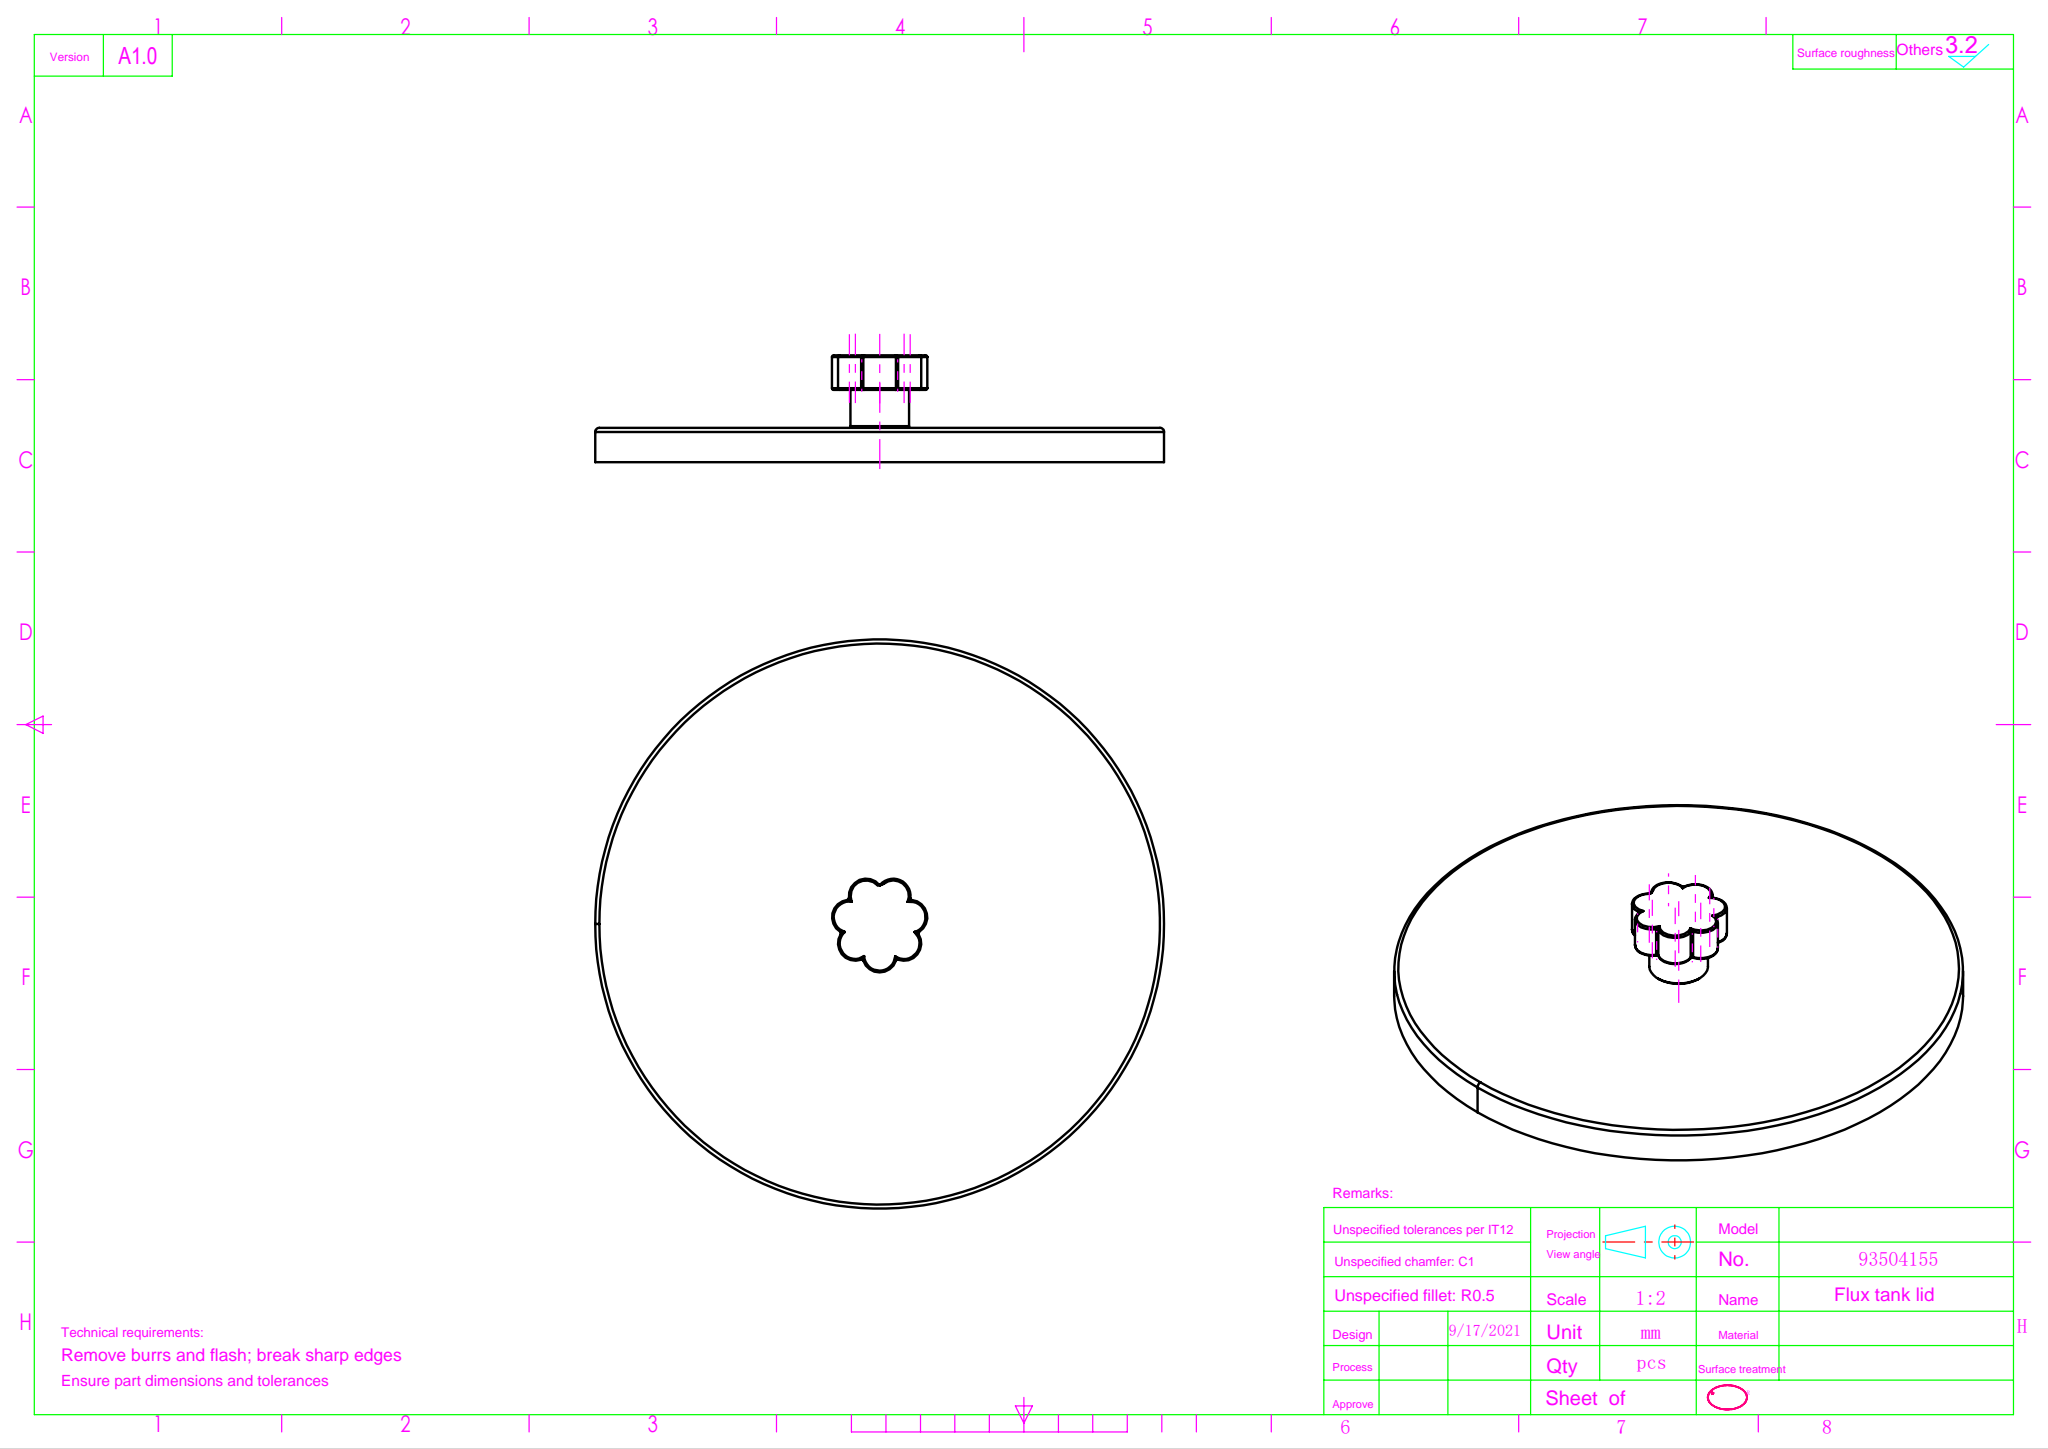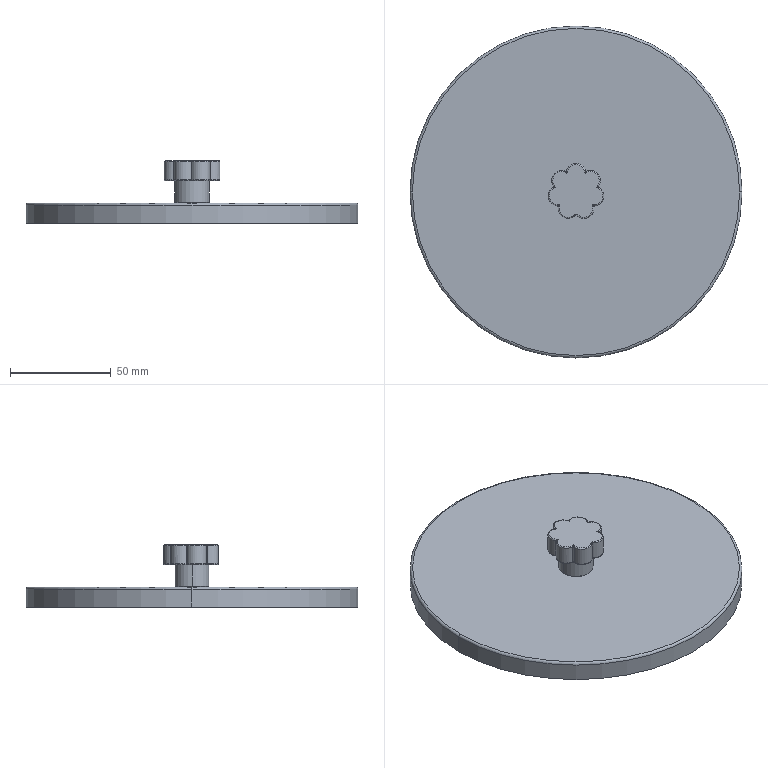Part | SolidWorks | 3 solids | 100 faces | box 165 x 165 x 31 mm | volume 59281 mm3 | cylinder 55 | spline 30 | plane 9 | torus 4 | cone 2 | commonest cylinder face diameters 6 x22 10 x10 1 x9 7 x4 17 x2 22.5 x2